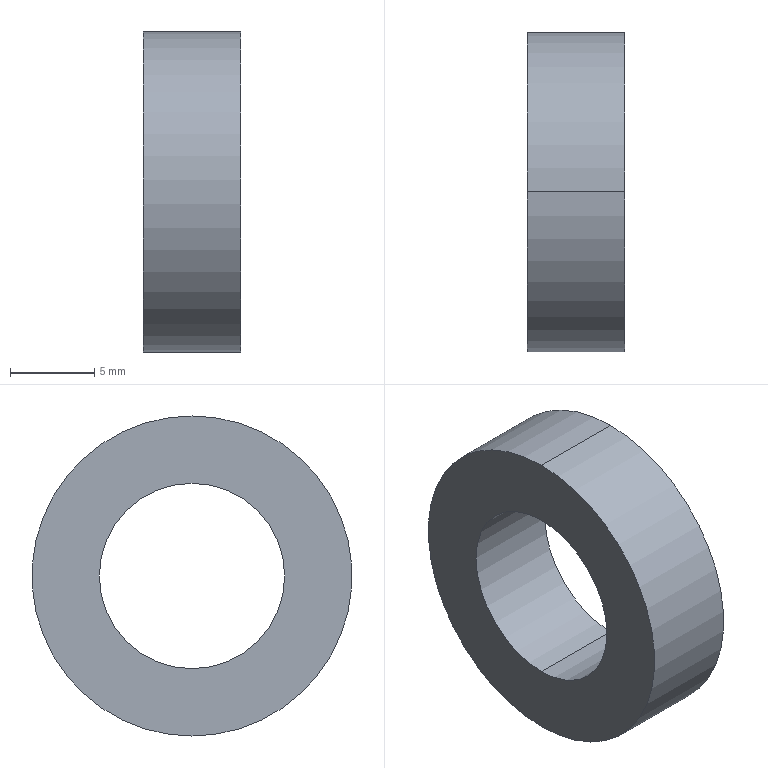Part | SolidWorks | features BaseBody 1 | 1 solid | 6 faces | box 5.8 x 19 x 19 mm | volume 1093 mm3 | cylinder 4 | plane 2 | commonest cylinder face diameters 11 x2 19 x2
STEP:
#1=CARTESIAN_POINT('',(3.237,1.896,-187.05));
#2=VERTEX_POINT('',#1);
#3=CARTESIAN_POINT('',(3.237,1.896,-206.05));
#4=VERTEX_POINT('',#3);
#5=CARTESIAN_POINT('',(3.237,1.896,-196.55));
#6=DIRECTION('',(-1.,0.,0.));
#7=DIRECTION('',(0.,0.,1.));
#8=AXIS2_PLACEMENT_3D('',#5,#6,#7);
#9=CIRCLE('',#8,9.5);
#10=EDGE_CURVE('',#2,#4,#9,.T.);
#11=ORIENTED_EDGE('',*,*,#10,.F.);
#12=CARTESIAN_POINT('',(9.037,1.896,-187.05));
#13=VERTEX_POINT('',#12);
#14=CARTESIAN_POINT('',(3.237,1.896,-187.05));
#15=DIRECTION('',(1.,0.,0.));
#16=VECTOR('',#15,1000.);
#17=LINE('',#14,#16);
#18=EDGE_CURVE('',#2,#13,#17,.T.);
#19=ORIENTED_EDGE('',*,*,#18,.T.);
#20=CARTESIAN_POINT('',(9.037,1.896,-206.05));
#21=VERTEX_POINT('',#20);
#22=CARTESIAN_POINT('',(9.037,1.896,-196.55));
#23=DIRECTION('',(-1.,0.,0.));
#24=DIRECTION('',(0.,0.,1.));
#25=AXIS2_PLACEMENT_3D('',#22,#23,#24);
#26=CIRCLE('',#25,9.5);
#27=EDGE_CURVE('',#13,#21,#26,.T.);
#28=ORIENTED_EDGE('',*,*,#27,.T.);
#29=CARTESIAN_POINT('',(3.237,1.896,-206.05));
#30=DIRECTION('',(1.,0.,0.));
#31=VECTOR('',#30,1000.);
#32=LINE('',#29,#31);
#33=EDGE_CURVE('',#4,#21,#32,.T.);
#34=ORIENTED_EDGE('',*,*,#33,.F.);
#35=EDGE_LOOP('',(#11,#19,#28,#34));
#36=FACE_OUTER_BOUND('',#35,.T.);
#37=CARTESIAN_POINT('',(3.237,1.896,-196.55));
#38=DIRECTION('',(1.,0.,0.));
#39=DIRECTION('',(0.,0.,-1.));
#40=AXIS2_PLACEMENT_3D('',#37,#38,#39);
#41=CYLINDRICAL_SURFACE('',#40,9.5);
#42=ADVANCED_FACE('',(#36),#41,.T.);
#43=CARTESIAN_POINT('',(3.237,1.896,-202.05));
#44=VERTEX_POINT('',#43);
#45=CARTESIAN_POINT('',(3.237,1.896,-191.05));
#46=VERTEX_POINT('',#45);
#47=CARTESIAN_POINT('',(3.237,1.896,-196.55));
#48=DIRECTION('',(-1.,0.,0.));
#49=DIRECTION('',(0.,0.,1.));
#50=AXIS2_PLACEMENT_3D('',#47,#48,#49);
#51=CIRCLE('',#50,5.5);
#52=EDGE_CURVE('',#44,#46,#51,.T.);
#53=ORIENTED_EDGE('',*,*,#52,.T.);
#54=CARTESIAN_POINT('',(9.037,1.896,-191.05));
#55=VERTEX_POINT('',#54);
#56=CARTESIAN_POINT('',(3.237,1.896,-191.05));
#57=DIRECTION('',(1.,0.,0.));
#58=VECTOR('',#57,1000.);
#59=LINE('',#56,#58);
#60=EDGE_CURVE('',#46,#55,#59,.T.);
#61=ORIENTED_EDGE('',*,*,#60,.T.);
#62=CARTESIAN_POINT('',(9.037,1.896,-202.05));
#63=VERTEX_POINT('',#62);
#64=CARTESIAN_POINT('',(9.037,1.896,-196.55));
#65=DIRECTION('',(-1.,0.,0.));
#66=DIRECTION('',(0.,0.,1.));
#67=AXIS2_PLACEMENT_3D('',#64,#65,#66);
#68=CIRCLE('',#67,5.5);
#69=EDGE_CURVE('',#63,#55,#68,.T.);
#70=ORIENTED_EDGE('',*,*,#69,.F.);
#71=CARTESIAN_POINT('',(3.237,1.896,-202.05));
#72=DIRECTION('',(1.,0.,0.));
#73=VECTOR('',#72,1000.);
#74=LINE('',#71,#73);
#75=EDGE_CURVE('',#44,#63,#74,.T.);
#76=ORIENTED_EDGE('',*,*,#75,.F.);
#77=EDGE_LOOP('',(#53,#61,#70,#76));
#78=FACE_OUTER_BOUND('',#77,.T.);
#79=CARTESIAN_POINT('',(3.237,1.896,-196.55));
#80=DIRECTION('',(1.,0.,0.));
#81=DIRECTION('',(0.,0.,-1.));
#82=AXIS2_PLACEMENT_3D('',#79,#80,#81);
#83=CYLINDRICAL_SURFACE('',#82,5.5);
#84=ADVANCED_FACE('',(#78),#83,.F.);
#85=ORIENTED_EDGE('',*,*,#60,.F.);
#86=CARTESIAN_POINT('',(3.237,1.896,-196.55));
#87=DIRECTION('',(-1.,0.,0.));
#88=DIRECTION('',(0.,0.,1.));
#89=AXIS2_PLACEMENT_3D('',#86,#87,#88);
#90=CIRCLE('',#89,5.5);
#91=EDGE_CURVE('',#46,#44,#90,.T.);
#92=ORIENTED_EDGE('',*,*,#91,.T.);
#93=ORIENTED_EDGE('',*,*,#75,.T.);
#94=CARTESIAN_POINT('',(9.037,1.896,-196.55));
#95=DIRECTION('',(-1.,0.,0.));
#96=DIRECTION('',(0.,0.,1.));
#97=AXIS2_PLACEMENT_3D('',#94,#95,#96);
#98=CIRCLE('',#97,5.5);
#99=EDGE_CURVE('',#55,#63,#98,.T.);
#100=ORIENTED_EDGE('',*,*,#99,.F.);
#101=EDGE_LOOP('',(#85,#92,#93,#100));
#102=FACE_OUTER_BOUND('',#101,.T.);
#103=CARTESIAN_POINT('',(3.237,1.896,-196.55));
#104=DIRECTION('',(1.,0.,0.));
#105=DIRECTION('',(0.,0.,-1.));
#106=AXIS2_PLACEMENT_3D('',#103,#104,#105);
#107=CYLINDRICAL_SURFACE('',#106,5.5);
#108=ADVANCED_FACE('',(#102),#107,.F.);
#109=ORIENTED_EDGE('',*,*,#18,.F.);
#110=CARTESIAN_POINT('',(3.237,1.896,-196.55));
#111=DIRECTION('',(-1.,0.,0.));
#112=DIRECTION('',(0.,0.,1.));
#113=AXIS2_PLACEMENT_3D('',#110,#111,#112);
#114=CIRCLE('',#113,9.5);
#115=EDGE_CURVE('',#4,#2,#114,.T.);
#116=ORIENTED_EDGE('',*,*,#115,.F.);
#117=ORIENTED_EDGE('',*,*,#33,.T.);
#118=CARTESIAN_POINT('',(9.037,1.896,-196.55));
#119=DIRECTION('',(-1.,0.,0.));
#120=DIRECTION('',(0.,0.,1.));
#121=AXIS2_PLACEMENT_3D('',#118,#119,#120);
#122=CIRCLE('',#121,9.5);
#123=EDGE_CURVE('',#21,#13,#122,.T.);
#124=ORIENTED_EDGE('',*,*,#123,.T.);
#125=EDGE_LOOP('',(#109,#116,#117,#124));
#126=FACE_OUTER_BOUND('',#125,.T.);
#127=CARTESIAN_POINT('',(3.237,1.896,-196.55));
#128=DIRECTION('',(1.,0.,0.));
#129=DIRECTION('',(0.,0.,-1.));
#130=AXIS2_PLACEMENT_3D('',#127,#128,#129);
#131=CYLINDRICAL_SURFACE('',#130,9.5);
#132=ADVANCED_FACE('',(#126),#131,.T.);
#133=ORIENTED_EDGE('',*,*,#69,.T.);
#134=ORIENTED_EDGE('',*,*,#99,.T.);
#135=EDGE_LOOP('',(#133,#134));
#136=FACE_BOUND('',#135,.T.);
#137=ORIENTED_EDGE('',*,*,#123,.F.);
#138=ORIENTED_EDGE('',*,*,#27,.F.);
#139=EDGE_LOOP('',(#137,#138));
#140=FACE_OUTER_BOUND('',#139,.T.);
#141=CARTESIAN_POINT('',(9.037,1.896,-196.55));
#142=DIRECTION('',(-1.,0.,0.));
#143=DIRECTION('',(0.,1.,0.));
#144=AXIS2_PLACEMENT_3D('',#141,#142,#143);
#145=PLANE('',#144);
#146=ADVANCED_FACE('',(#136,#140),#145,.F.);
#147=ORIENTED_EDGE('',*,*,#52,.F.);
#148=ORIENTED_EDGE('',*,*,#91,.F.);
#149=EDGE_LOOP('',(#147,#148));
#150=FACE_BOUND('',#149,.T.);
#151=ORIENTED_EDGE('',*,*,#115,.T.);
#152=ORIENTED_EDGE('',*,*,#10,.T.);
#153=EDGE_LOOP('',(#151,#152));
#154=FACE_OUTER_BOUND('',#153,.T.);
#155=CARTESIAN_POINT('',(3.237,1.896,-196.55));
#156=DIRECTION('',(-1.,0.,0.));
#157=DIRECTION('',(0.,1.,0.));
#158=AXIS2_PLACEMENT_3D('',#155,#156,#157);
#159=PLANE('',#158);
#160=ADVANCED_FACE('',(#150,#154),#159,.T.);
#161=CLOSED_SHELL('',(#42,#84,#108,#132,#146,#160));
#162=MANIFOLD_SOLID_BREP('',#161);
#163=CARTESIAN_POINT('',(0.,0.,0.));
#164=DIRECTION('',(0.,0.,1.));
#165=DIRECTION('',(1.,0.,0.));
#166=AXIS2_PLACEMENT_3D('',#163,#164,#165);
#167=(LENGTH_UNIT()NAMED_UNIT(*)SI_UNIT(.MILLI.,.METRE.));
#168=UNCERTAINTY_MEASURE_WITH_UNIT(LENGTH_MEASURE(0.00001),#167,'','');
#169=(NAMED_UNIT(*)PLANE_ANGLE_UNIT()SI_UNIT($,.RADIAN.));
#170=(NAMED_UNIT(*)SI_UNIT($,.STERADIAN.)SOLID_ANGLE_UNIT());
#171=(GEOMETRIC_REPRESENTATION_CONTEXT(3)GLOBAL_UNCERTAINTY_ASSIGNED_CONTEXT((#168))GLOBAL_UNIT_ASSIGNED_CONTEXT((#167,#169,#170))REPRESENTATION_CONTEXT('',''));
#172=ADVANCED_BREP_SHAPE_REPRESENTATION('',(#162,#166),#171);